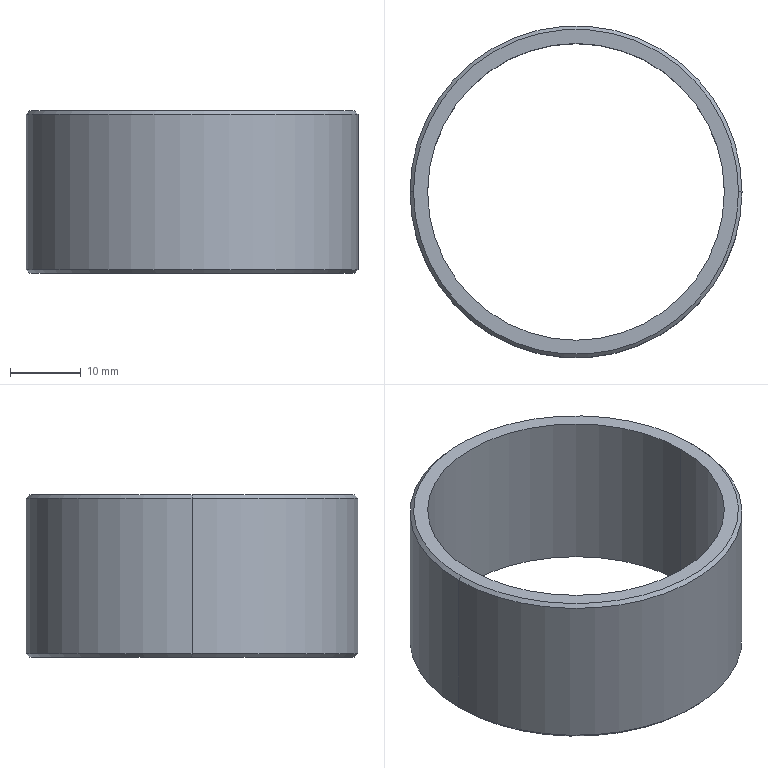Part | SolidWorks | features Chamfer 1, Extrusion 1 | 1 solid | 10 faces | box 47 x 47 x 23 mm | volume 8002 mm3 | cone 4 | cylinder 4 | plane 2 | commonest cylinder face diameters 42 x2 47 x2
STEP:
#1=CARTESIAN_POINT('',(-23.,0.,0.));
#2=VERTEX_POINT('',#1);
#3=CARTESIAN_POINT('',(23.,0.,0.));
#4=VERTEX_POINT('',#3);
#5=CARTESIAN_POINT('',(0.,0.,0.));
#6=DIRECTION('',(0.,0.,-1.));
#7=DIRECTION('',(1.,0.,0.));
#8=AXIS2_PLACEMENT_3D('',#5,#6,#7);
#9=CIRCLE('',#8,23.);
#10=EDGE_CURVE('',#2,#4,#9,.T.);
#11=ORIENTED_EDGE('',*,*,#10,.F.);
#12=CARTESIAN_POINT('',(-23.5,0.,0.5));
#13=VERTEX_POINT('',#12);
#14=CARTESIAN_POINT('',(-23.5,0.,0.5));
#15=DIRECTION('',(-0.7071,0.,0.7071));
#16=VECTOR('',#15,1000.);
#17=LINE('',#14,#16);
#18=EDGE_CURVE('',#2,#13,#17,.T.);
#19=ORIENTED_EDGE('',*,*,#18,.T.);
#20=CARTESIAN_POINT('',(23.5,0.,0.5));
#21=VERTEX_POINT('',#20);
#22=CARTESIAN_POINT('',(0.,0.,0.5));
#23=DIRECTION('',(0.,0.,1.));
#24=DIRECTION('',(1.,0.,0.));
#25=AXIS2_PLACEMENT_3D('',#22,#23,#24);
#26=CIRCLE('',#25,23.5);
#27=EDGE_CURVE('',#21,#13,#26,.T.);
#28=ORIENTED_EDGE('',*,*,#27,.F.);
#29=CARTESIAN_POINT('',(23.5,0.,0.5));
#30=DIRECTION('',(0.7071,0.,0.7071));
#31=VECTOR('',#30,1000.);
#32=LINE('',#29,#31);
#33=EDGE_CURVE('',#4,#21,#32,.T.);
#34=ORIENTED_EDGE('',*,*,#33,.F.);
#35=EDGE_LOOP('',(#11,#19,#28,#34));
#36=FACE_OUTER_BOUND('',#35,.T.);
#37=CARTESIAN_POINT('',(0.,0.,0.5));
#38=DIRECTION('',(0.,0.,1.));
#39=DIRECTION('',(1.,0.,0.));
#40=AXIS2_PLACEMENT_3D('',#37,#38,#39);
#41=CONICAL_SURFACE('',#40,23.5,0.7854);
#42=ADVANCED_FACE('',(#36),#41,.T.);
#43=CARTESIAN_POINT('',(23.,0.,23.));
#44=VERTEX_POINT('',#43);
#45=CARTESIAN_POINT('',(-23.,0.,23.));
#46=VERTEX_POINT('',#45);
#47=CARTESIAN_POINT('',(0.,0.,23.));
#48=DIRECTION('',(0.,0.,1.));
#49=DIRECTION('',(1.,0.,0.));
#50=AXIS2_PLACEMENT_3D('',#47,#48,#49);
#51=CIRCLE('',#50,23.);
#52=EDGE_CURVE('',#44,#46,#51,.T.);
#53=ORIENTED_EDGE('',*,*,#52,.F.);
#54=CARTESIAN_POINT('',(23.5,0.,22.5));
#55=VERTEX_POINT('',#54);
#56=CARTESIAN_POINT('',(23.,0.,23.));
#57=DIRECTION('',(0.7071,0.,-0.7071));
#58=VECTOR('',#57,1000.);
#59=LINE('',#56,#58);
#60=EDGE_CURVE('',#44,#55,#59,.T.);
#61=ORIENTED_EDGE('',*,*,#60,.T.);
#62=CARTESIAN_POINT('',(-23.5,0.,22.5));
#63=VERTEX_POINT('',#62);
#64=CARTESIAN_POINT('',(0.,0.,22.5));
#65=DIRECTION('',(0.,0.,-1.));
#66=DIRECTION('',(1.,0.,0.));
#67=AXIS2_PLACEMENT_3D('',#64,#65,#66);
#68=CIRCLE('',#67,23.5);
#69=EDGE_CURVE('',#63,#55,#68,.T.);
#70=ORIENTED_EDGE('',*,*,#69,.F.);
#71=CARTESIAN_POINT('',(-23.,0.,23.));
#72=DIRECTION('',(-0.7071,0.,-0.7071));
#73=VECTOR('',#72,1000.);
#74=LINE('',#71,#73);
#75=EDGE_CURVE('',#46,#63,#74,.T.);
#76=ORIENTED_EDGE('',*,*,#75,.F.);
#77=EDGE_LOOP('',(#53,#61,#70,#76));
#78=FACE_OUTER_BOUND('',#77,.T.);
#79=CARTESIAN_POINT('',(0.,0.,23.));
#80=DIRECTION('',(0.,0.,-1.));
#81=DIRECTION('',(-1.,0.,0.));
#82=AXIS2_PLACEMENT_3D('',#79,#80,#81);
#83=CONICAL_SURFACE('',#82,23.,0.7854);
#84=ADVANCED_FACE('',(#78),#83,.T.);
#85=CARTESIAN_POINT('',(-21.,0.,23.));
#86=VERTEX_POINT('',#85);
#87=CARTESIAN_POINT('',(21.,0.,23.));
#88=VERTEX_POINT('',#87);
#89=CARTESIAN_POINT('',(0.,0.,23.));
#90=DIRECTION('',(0.,0.,1.));
#91=DIRECTION('',(1.,0.,0.));
#92=AXIS2_PLACEMENT_3D('',#89,#90,#91);
#93=CIRCLE('',#92,21.);
#94=EDGE_CURVE('',#86,#88,#93,.T.);
#95=ORIENTED_EDGE('',*,*,#94,.T.);
#96=CARTESIAN_POINT('',(21.,0.,0.));
#97=VERTEX_POINT('',#96);
#98=CARTESIAN_POINT('',(21.,0.,23.));
#99=DIRECTION('',(0.,0.,-1.));
#100=VECTOR('',#99,1000.);
#101=LINE('',#98,#100);
#102=EDGE_CURVE('',#88,#97,#101,.T.);
#103=ORIENTED_EDGE('',*,*,#102,.T.);
#104=CARTESIAN_POINT('',(-21.,0.,0.));
#105=VERTEX_POINT('',#104);
#106=CARTESIAN_POINT('',(0.,0.,0.));
#107=DIRECTION('',(0.,0.,1.));
#108=DIRECTION('',(1.,0.,0.));
#109=AXIS2_PLACEMENT_3D('',#106,#107,#108);
#110=CIRCLE('',#109,21.);
#111=EDGE_CURVE('',#105,#97,#110,.T.);
#112=ORIENTED_EDGE('',*,*,#111,.F.);
#113=CARTESIAN_POINT('',(-21.,0.,23.));
#114=DIRECTION('',(0.,0.,-1.));
#115=VECTOR('',#114,1000.);
#116=LINE('',#113,#115);
#117=EDGE_CURVE('',#86,#105,#116,.T.);
#118=ORIENTED_EDGE('',*,*,#117,.F.);
#119=EDGE_LOOP('',(#95,#103,#112,#118));
#120=FACE_OUTER_BOUND('',#119,.T.);
#121=CARTESIAN_POINT('',(0.,0.,23.));
#122=DIRECTION('',(0.,0.,-1.));
#123=DIRECTION('',(-1.,0.,0.));
#124=AXIS2_PLACEMENT_3D('',#121,#122,#123);
#125=CYLINDRICAL_SURFACE('',#124,21.);
#126=ADVANCED_FACE('',(#120),#125,.F.);
#127=ORIENTED_EDGE('',*,*,#69,.T.);
#128=CARTESIAN_POINT('',(23.5,0.,23.));
#129=DIRECTION('',(0.,0.,-1.));
#130=VECTOR('',#129,1000.);
#131=LINE('',#128,#130);
#132=EDGE_CURVE('',#55,#21,#131,.T.);
#133=ORIENTED_EDGE('',*,*,#132,.T.);
#134=ORIENTED_EDGE('',*,*,#27,.T.);
#135=CARTESIAN_POINT('',(-23.5,0.,23.));
#136=DIRECTION('',(0.,0.,-1.));
#137=VECTOR('',#136,1000.);
#138=LINE('',#135,#137);
#139=EDGE_CURVE('',#63,#13,#138,.T.);
#140=ORIENTED_EDGE('',*,*,#139,.F.);
#141=EDGE_LOOP('',(#127,#133,#134,#140));
#142=FACE_OUTER_BOUND('',#141,.T.);
#143=CARTESIAN_POINT('',(0.,0.,23.));
#144=DIRECTION('',(0.,0.,-1.));
#145=DIRECTION('',(-1.,0.,0.));
#146=AXIS2_PLACEMENT_3D('',#143,#144,#145);
#147=CYLINDRICAL_SURFACE('',#146,23.5);
#148=ADVANCED_FACE('',(#142),#147,.T.);
#149=CARTESIAN_POINT('',(0.,0.,23.));
#150=DIRECTION('',(0.,0.,1.));
#151=DIRECTION('',(1.,0.,0.));
#152=AXIS2_PLACEMENT_3D('',#149,#150,#151);
#153=CIRCLE('',#152,23.);
#154=EDGE_CURVE('',#46,#44,#153,.T.);
#155=ORIENTED_EDGE('',*,*,#154,.T.);
#156=ORIENTED_EDGE('',*,*,#52,.T.);
#157=EDGE_LOOP('',(#155,#156));
#158=FACE_OUTER_BOUND('',#157,.T.);
#159=ORIENTED_EDGE('',*,*,#94,.F.);
#160=CARTESIAN_POINT('',(0.,0.,23.));
#161=DIRECTION('',(0.,0.,1.));
#162=DIRECTION('',(1.,0.,0.));
#163=AXIS2_PLACEMENT_3D('',#160,#161,#162);
#164=CIRCLE('',#163,21.);
#165=EDGE_CURVE('',#88,#86,#164,.T.);
#166=ORIENTED_EDGE('',*,*,#165,.F.);
#167=EDGE_LOOP('',(#159,#166));
#168=FACE_BOUND('',#167,.T.);
#169=CARTESIAN_POINT('',(0.,0.,23.));
#170=DIRECTION('',(0.,0.,1.));
#171=DIRECTION('',(1.,0.,0.));
#172=AXIS2_PLACEMENT_3D('',#169,#170,#171);
#173=PLANE('',#172);
#174=ADVANCED_FACE('',(#158,#168),#173,.T.);
#175=CARTESIAN_POINT('',(0.,0.,0.));
#176=DIRECTION('',(0.,0.,-1.));
#177=DIRECTION('',(1.,0.,0.));
#178=AXIS2_PLACEMENT_3D('',#175,#176,#177);
#179=CIRCLE('',#178,23.);
#180=EDGE_CURVE('',#4,#2,#179,.T.);
#181=ORIENTED_EDGE('',*,*,#180,.T.);
#182=ORIENTED_EDGE('',*,*,#10,.T.);
#183=EDGE_LOOP('',(#181,#182));
#184=FACE_OUTER_BOUND('',#183,.T.);
#185=ORIENTED_EDGE('',*,*,#111,.T.);
#186=CARTESIAN_POINT('',(0.,0.,0.));
#187=DIRECTION('',(0.,0.,1.));
#188=DIRECTION('',(1.,0.,0.));
#189=AXIS2_PLACEMENT_3D('',#186,#187,#188);
#190=CIRCLE('',#189,21.);
#191=EDGE_CURVE('',#97,#105,#190,.T.);
#192=ORIENTED_EDGE('',*,*,#191,.T.);
#193=EDGE_LOOP('',(#185,#192));
#194=FACE_BOUND('',#193,.T.);
#195=CARTESIAN_POINT('',(0.,0.,0.));
#196=DIRECTION('',(0.,0.,1.));
#197=DIRECTION('',(1.,0.,0.));
#198=AXIS2_PLACEMENT_3D('',#195,#196,#197);
#199=PLANE('',#198);
#200=ADVANCED_FACE('',(#184,#194),#199,.F.);
#201=ORIENTED_EDGE('',*,*,#132,.F.);
#202=CARTESIAN_POINT('',(0.,0.,22.5));
#203=DIRECTION('',(0.,0.,-1.));
#204=DIRECTION('',(1.,0.,0.));
#205=AXIS2_PLACEMENT_3D('',#202,#203,#204);
#206=CIRCLE('',#205,23.5);
#207=EDGE_CURVE('',#55,#63,#206,.T.);
#208=ORIENTED_EDGE('',*,*,#207,.T.);
#209=ORIENTED_EDGE('',*,*,#139,.T.);
#210=CARTESIAN_POINT('',(0.,0.,0.5));
#211=DIRECTION('',(0.,0.,1.));
#212=DIRECTION('',(1.,0.,0.));
#213=AXIS2_PLACEMENT_3D('',#210,#211,#212);
#214=CIRCLE('',#213,23.5);
#215=EDGE_CURVE('',#13,#21,#214,.T.);
#216=ORIENTED_EDGE('',*,*,#215,.T.);
#217=EDGE_LOOP('',(#201,#208,#209,#216));
#218=FACE_OUTER_BOUND('',#217,.T.);
#219=CARTESIAN_POINT('',(0.,0.,23.));
#220=DIRECTION('',(0.,0.,-1.));
#221=DIRECTION('',(-1.,0.,0.));
#222=AXIS2_PLACEMENT_3D('',#219,#220,#221);
#223=CYLINDRICAL_SURFACE('',#222,23.5);
#224=ADVANCED_FACE('',(#218),#223,.T.);
#225=ORIENTED_EDGE('',*,*,#102,.F.);
#226=ORIENTED_EDGE('',*,*,#165,.T.);
#227=ORIENTED_EDGE('',*,*,#117,.T.);
#228=ORIENTED_EDGE('',*,*,#191,.F.);
#229=EDGE_LOOP('',(#225,#226,#227,#228));
#230=FACE_OUTER_BOUND('',#229,.T.);
#231=CARTESIAN_POINT('',(0.,0.,23.));
#232=DIRECTION('',(0.,0.,-1.));
#233=DIRECTION('',(-1.,0.,0.));
#234=AXIS2_PLACEMENT_3D('',#231,#232,#233);
#235=CYLINDRICAL_SURFACE('',#234,21.);
#236=ADVANCED_FACE('',(#230),#235,.F.);
#237=ORIENTED_EDGE('',*,*,#60,.F.);
#238=ORIENTED_EDGE('',*,*,#154,.F.);
#239=ORIENTED_EDGE('',*,*,#75,.T.);
#240=ORIENTED_EDGE('',*,*,#207,.F.);
#241=EDGE_LOOP('',(#237,#238,#239,#240));
#242=FACE_OUTER_BOUND('',#241,.T.);
#243=CARTESIAN_POINT('',(0.,0.,23.));
#244=DIRECTION('',(0.,0.,-1.));
#245=DIRECTION('',(-1.,0.,0.));
#246=AXIS2_PLACEMENT_3D('',#243,#244,#245);
#247=CONICAL_SURFACE('',#246,23.,0.7854);
#248=ADVANCED_FACE('',(#242),#247,.T.);
#249=ORIENTED_EDGE('',*,*,#18,.F.);
#250=ORIENTED_EDGE('',*,*,#180,.F.);
#251=ORIENTED_EDGE('',*,*,#33,.T.);
#252=ORIENTED_EDGE('',*,*,#215,.F.);
#253=EDGE_LOOP('',(#249,#250,#251,#252));
#254=FACE_OUTER_BOUND('',#253,.T.);
#255=CARTESIAN_POINT('',(0.,0.,0.5));
#256=DIRECTION('',(0.,0.,1.));
#257=DIRECTION('',(1.,0.,0.));
#258=AXIS2_PLACEMENT_3D('',#255,#256,#257);
#259=CONICAL_SURFACE('',#258,23.5,0.7854);
#260=ADVANCED_FACE('',(#254),#259,.T.);
#261=CLOSED_SHELL('',(#42,#84,#126,#148,#174,#200,#224,#236,#248,#260));
#262=MANIFOLD_SOLID_BREP('',#261);
#263=CARTESIAN_POINT('',(0.,0.,0.));
#264=DIRECTION('',(0.,0.,1.));
#265=DIRECTION('',(1.,0.,0.));
#266=AXIS2_PLACEMENT_3D('',#263,#264,#265);
#267=(LENGTH_UNIT()NAMED_UNIT(*)SI_UNIT(.MILLI.,.METRE.));
#268=UNCERTAINTY_MEASURE_WITH_UNIT(LENGTH_MEASURE(0.00001),#267,'','');
#269=(NAMED_UNIT(*)PLANE_ANGLE_UNIT()SI_UNIT($,.RADIAN.));
#270=(NAMED_UNIT(*)SI_UNIT($,.STERADIAN.)SOLID_ANGLE_UNIT());
#271=(GEOMETRIC_REPRESENTATION_CONTEXT(3)GLOBAL_UNCERTAINTY_ASSIGNED_CONTEXT((#268))GLOBAL_UNIT_ASSIGNED_CONTEXT((#267,#269,#270))REPRESENTATION_CONTEXT('',''));
#272=ADVANCED_BREP_SHAPE_REPRESENTATION('',(#262,#266),#271);